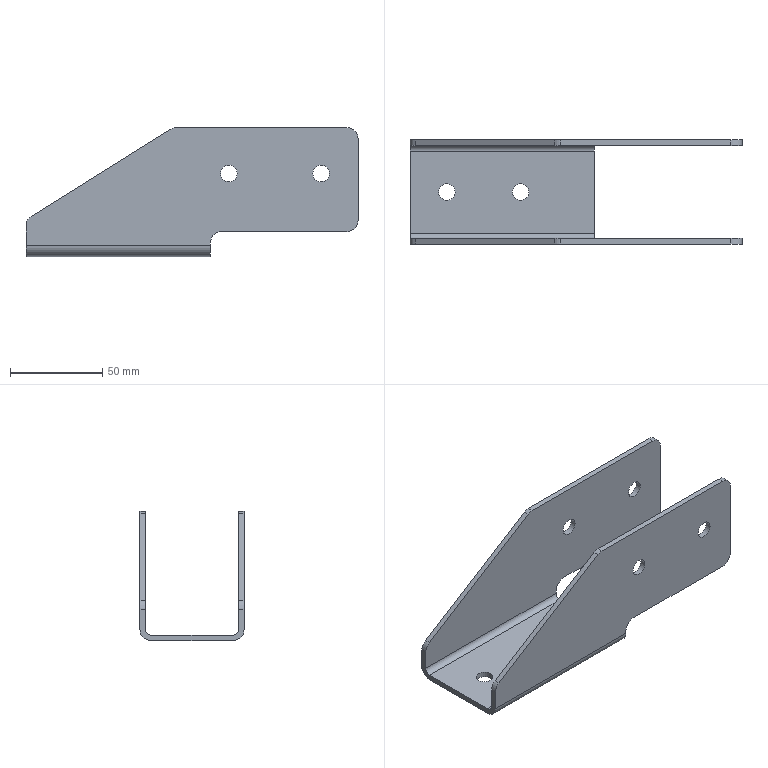Part | STEP file | Leg support-05 | 1 solid | 36 faces | box 180 x 56.5 x 70 mm | volume 69908 mm3 | cylinder 14 | plane 14 | spline 8 | commonest cylinder face diameters 12 x12 6 x2